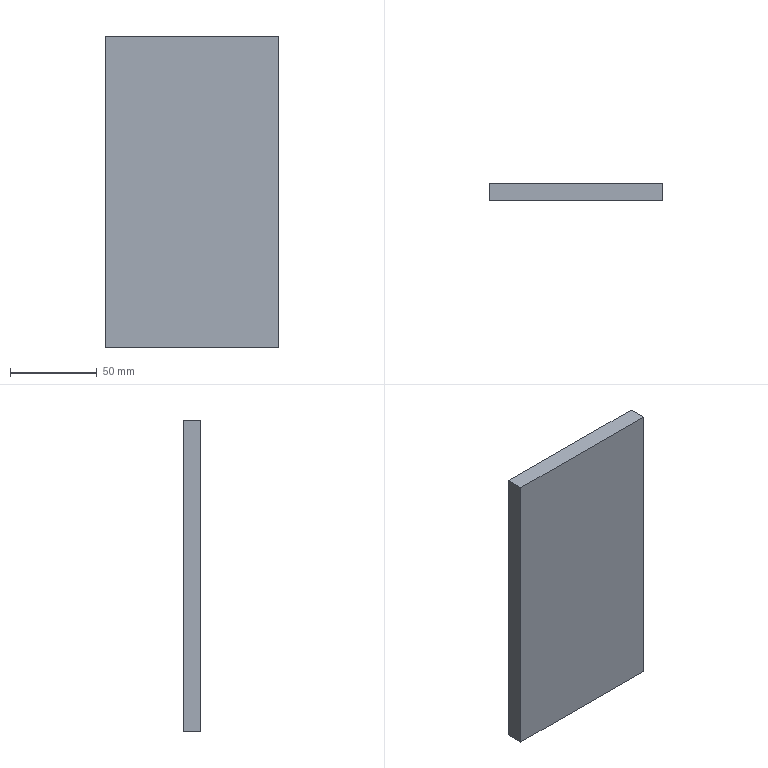Part | STEP file | A14-055 | 1 solid | 6 faces | box 100 x 10 x 180 mm | volume 180000 mm3 | plane 6
STEP:
#1=CARTESIAN_POINT('',(0.,0.,0.));
#2=DIRECTION('',(0.,0.,1.));
#3=DIRECTION('',(1.,0.,0.));
#4=AXIS2_PLACEMENT_3D('',#1,#2,#3);
#5=CARTESIAN_POINT('',(50.,-5.,90.));
#6=VERTEX_POINT('',#5);
#7=CARTESIAN_POINT('',(50.,-5.,-90.));
#8=VERTEX_POINT('',#7);
#9=CARTESIAN_POINT('',(50.,-5.,-90.));
#10=DIRECTION('',(0.,0.,-1.));
#11=VECTOR('',#10,1.);
#12=LINE('',#9,#11);
#13=CARTESIAN_POINT('',(50.,5.,-90.));
#14=DIRECTION('',(-1.,0.,0.));
#15=DIRECTION('',(0.,0.,1.));
#16=AXIS2_PLACEMENT_3D('',#13,#14,#15);
#17=PLANE('',#16);
#18=CARTESIAN_POINT('',(0.,-10.));
#19=DIRECTION('',(-1.,0.));
#20=VECTOR('',#19,1.);
#21=LINE('',#18,#20);
#22=(GEOMETRIC_REPRESENTATION_CONTEXT(2)PARAMETRIC_REPRESENTATION_CONTEXT()REPRESENTATION_CONTEXT('',''));
#23=DEFINITIONAL_REPRESENTATION('',(#21),#22);
#24=PCURVE('',#17,#23);
#25=CARTESIAN_POINT('',(0.,-5.,0.));
#26=DIRECTION('',(0.,1.,0.));
#27=DIRECTION('',(0.,0.,1.));
#28=AXIS2_PLACEMENT_3D('',#25,#26,#27);
#29=PLANE('',#28);
#30=CARTESIAN_POINT('',(-90.,50.));
#31=DIRECTION('',(-1.,0.));
#32=VECTOR('',#31,1.);
#33=LINE('',#30,#32);
#34=(GEOMETRIC_REPRESENTATION_CONTEXT(2)PARAMETRIC_REPRESENTATION_CONTEXT()REPRESENTATION_CONTEXT('',''));
#35=DEFINITIONAL_REPRESENTATION('',(#33),#34);
#36=PCURVE('',#29,#35);
#37=SURFACE_CURVE('',#12,(#24,#36),.PCURVE_S1.);
#38=EDGE_CURVE('',#6,#8,#37,.T.);
#39=ORIENTED_EDGE('',*,*,#38,.T.);
#40=CARTESIAN_POINT('',(50.,5.,-90.));
#41=VERTEX_POINT('',#40);
#42=CARTESIAN_POINT('',(50.,5.,-90.));
#43=DIRECTION('',(0.,-1.,0.));
#44=VECTOR('',#43,1.);
#45=LINE('',#42,#44);
#46=CARTESIAN_POINT('',(0.,0.));
#47=DIRECTION('',(0.,-1.));
#48=VECTOR('',#47,1.);
#49=LINE('',#46,#48);
#50=(GEOMETRIC_REPRESENTATION_CONTEXT(2)PARAMETRIC_REPRESENTATION_CONTEXT()REPRESENTATION_CONTEXT('',''));
#51=DEFINITIONAL_REPRESENTATION('',(#49),#50);
#52=PCURVE('',#17,#51);
#53=CARTESIAN_POINT('',(-50.,5.,-90.));
#54=DIRECTION('',(0.,0.,1.));
#55=DIRECTION('',(1.,0.,0.));
#56=AXIS2_PLACEMENT_3D('',#53,#54,#55);
#57=PLANE('',#56);
#58=CARTESIAN_POINT('',(100.,0.));
#59=DIRECTION('',(0.,-1.));
#60=VECTOR('',#59,1.);
#61=LINE('',#58,#60);
#62=(GEOMETRIC_REPRESENTATION_CONTEXT(2)PARAMETRIC_REPRESENTATION_CONTEXT()REPRESENTATION_CONTEXT('',''));
#63=DEFINITIONAL_REPRESENTATION('',(#61),#62);
#64=PCURVE('',#57,#63);
#65=SURFACE_CURVE('',#45,(#52,#64),.PCURVE_S1.);
#66=EDGE_CURVE('',#41,#8,#65,.T.);
#67=ORIENTED_EDGE('',*,*,#66,.F.);
#68=CARTESIAN_POINT('',(50.,5.,90.));
#69=VERTEX_POINT('',#68);
#70=CARTESIAN_POINT('',(50.,5.,-90.));
#71=DIRECTION('',(0.,0.,-1.));
#72=VECTOR('',#71,1.);
#73=LINE('',#70,#72);
#74=CARTESIAN_POINT('',(0.,0.));
#75=DIRECTION('',(-1.,0.));
#76=VECTOR('',#75,1.);
#77=LINE('',#74,#76);
#78=(GEOMETRIC_REPRESENTATION_CONTEXT(2)PARAMETRIC_REPRESENTATION_CONTEXT()REPRESENTATION_CONTEXT('',''));
#79=DEFINITIONAL_REPRESENTATION('',(#77),#78);
#80=PCURVE('',#17,#79);
#81=CARTESIAN_POINT('',(0.,5.,0.));
#82=DIRECTION('',(0.,1.,0.));
#83=DIRECTION('',(0.,0.,1.));
#84=AXIS2_PLACEMENT_3D('',#81,#82,#83);
#85=PLANE('',#84);
#86=CARTESIAN_POINT('',(-90.,50.));
#87=DIRECTION('',(-1.,0.));
#88=VECTOR('',#87,1.);
#89=LINE('',#86,#88);
#90=(GEOMETRIC_REPRESENTATION_CONTEXT(2)PARAMETRIC_REPRESENTATION_CONTEXT()REPRESENTATION_CONTEXT('',''));
#91=DEFINITIONAL_REPRESENTATION('',(#89),#90);
#92=PCURVE('',#85,#91);
#93=SURFACE_CURVE('',#73,(#80,#92),.PCURVE_S1.);
#94=EDGE_CURVE('',#69,#41,#93,.T.);
#95=ORIENTED_EDGE('',*,*,#94,.F.);
#96=CARTESIAN_POINT('',(50.,5.,90.));
#97=DIRECTION('',(0.,-1.,0.));
#98=VECTOR('',#97,1.);
#99=LINE('',#96,#98);
#100=CARTESIAN_POINT('',(180.,0.));
#101=DIRECTION('',(0.,-1.));
#102=VECTOR('',#101,1.);
#103=LINE('',#100,#102);
#104=(GEOMETRIC_REPRESENTATION_CONTEXT(2)PARAMETRIC_REPRESENTATION_CONTEXT()REPRESENTATION_CONTEXT('',''));
#105=DEFINITIONAL_REPRESENTATION('',(#103),#104);
#106=PCURVE('',#17,#105);
#107=CARTESIAN_POINT('',(-50.,5.,90.));
#108=DIRECTION('',(0.,0.,-1.));
#109=DIRECTION('',(-1.,0.,0.));
#110=AXIS2_PLACEMENT_3D('',#107,#108,#109);
#111=PLANE('',#110);
#112=CARTESIAN_POINT('',(-100.,0.));
#113=DIRECTION('',(0.,-1.));
#114=VECTOR('',#113,1.);
#115=LINE('',#112,#114);
#116=(GEOMETRIC_REPRESENTATION_CONTEXT(2)PARAMETRIC_REPRESENTATION_CONTEXT()REPRESENTATION_CONTEXT('',''));
#117=DEFINITIONAL_REPRESENTATION('',(#115),#116);
#118=PCURVE('',#111,#117);
#119=SURFACE_CURVE('',#99,(#106,#118),.PCURVE_S1.);
#120=EDGE_CURVE('',#69,#6,#119,.T.);
#121=ORIENTED_EDGE('',*,*,#120,.T.);
#122=EDGE_LOOP('',(#39,#67,#95,#121));
#123=FACE_BOUND('',#122,.T.);
#124=ADVANCED_FACE('',(#123),#17,.F.);
#125=CARTESIAN_POINT('',(-50.,-5.,-90.));
#126=VERTEX_POINT('',#125);
#127=CARTESIAN_POINT('',(-50.,-5.,-90.));
#128=DIRECTION('',(-1.,0.,0.));
#129=VECTOR('',#128,1.);
#130=LINE('',#127,#129);
#131=CARTESIAN_POINT('',(0.,-10.));
#132=DIRECTION('',(-1.,0.));
#133=VECTOR('',#132,1.);
#134=LINE('',#131,#133);
#135=(GEOMETRIC_REPRESENTATION_CONTEXT(2)PARAMETRIC_REPRESENTATION_CONTEXT()REPRESENTATION_CONTEXT('',''));
#136=DEFINITIONAL_REPRESENTATION('',(#134),#135);
#137=PCURVE('',#57,#136);
#138=CARTESIAN_POINT('',(-90.,-50.));
#139=DIRECTION('',(0.,-1.));
#140=VECTOR('',#139,1.);
#141=LINE('',#138,#140);
#142=(GEOMETRIC_REPRESENTATION_CONTEXT(2)PARAMETRIC_REPRESENTATION_CONTEXT()REPRESENTATION_CONTEXT('',''));
#143=DEFINITIONAL_REPRESENTATION('',(#141),#142);
#144=PCURVE('',#29,#143);
#145=SURFACE_CURVE('',#130,(#137,#144),.PCURVE_S1.);
#146=EDGE_CURVE('',#8,#126,#145,.T.);
#147=ORIENTED_EDGE('',*,*,#146,.T.);
#148=CARTESIAN_POINT('',(-50.,5.,-90.));
#149=VERTEX_POINT('',#148);
#150=CARTESIAN_POINT('',(-50.,5.,-90.));
#151=DIRECTION('',(0.,-1.,0.));
#152=VECTOR('',#151,1.);
#153=LINE('',#150,#152);
#154=CARTESIAN_POINT('',(0.,0.));
#155=DIRECTION('',(0.,-1.));
#156=VECTOR('',#155,1.);
#157=LINE('',#154,#156);
#158=(GEOMETRIC_REPRESENTATION_CONTEXT(2)PARAMETRIC_REPRESENTATION_CONTEXT()REPRESENTATION_CONTEXT('',''));
#159=DEFINITIONAL_REPRESENTATION('',(#157),#158);
#160=PCURVE('',#57,#159);
#161=CARTESIAN_POINT('',(-50.,5.,-90.));
#162=DIRECTION('',(1.,0.,0.));
#163=DIRECTION('',(0.,0.,-1.));
#164=AXIS2_PLACEMENT_3D('',#161,#162,#163);
#165=PLANE('',#164);
#166=CARTESIAN_POINT('',(0.,0.));
#167=DIRECTION('',(0.,-1.));
#168=VECTOR('',#167,1.);
#169=LINE('',#166,#168);
#170=(GEOMETRIC_REPRESENTATION_CONTEXT(2)PARAMETRIC_REPRESENTATION_CONTEXT()REPRESENTATION_CONTEXT('',''));
#171=DEFINITIONAL_REPRESENTATION('',(#169),#170);
#172=PCURVE('',#165,#171);
#173=SURFACE_CURVE('',#153,(#160,#172),.PCURVE_S1.);
#174=EDGE_CURVE('',#149,#126,#173,.T.);
#175=ORIENTED_EDGE('',*,*,#174,.F.);
#176=CARTESIAN_POINT('',(-50.,5.,-90.));
#177=DIRECTION('',(-1.,0.,0.));
#178=VECTOR('',#177,1.);
#179=LINE('',#176,#178);
#180=CARTESIAN_POINT('',(0.,0.));
#181=DIRECTION('',(-1.,0.));
#182=VECTOR('',#181,1.);
#183=LINE('',#180,#182);
#184=(GEOMETRIC_REPRESENTATION_CONTEXT(2)PARAMETRIC_REPRESENTATION_CONTEXT()REPRESENTATION_CONTEXT('',''));
#185=DEFINITIONAL_REPRESENTATION('',(#183),#184);
#186=PCURVE('',#57,#185);
#187=CARTESIAN_POINT('',(-90.,-50.));
#188=DIRECTION('',(0.,-1.));
#189=VECTOR('',#188,1.);
#190=LINE('',#187,#189);
#191=(GEOMETRIC_REPRESENTATION_CONTEXT(2)PARAMETRIC_REPRESENTATION_CONTEXT()REPRESENTATION_CONTEXT('',''));
#192=DEFINITIONAL_REPRESENTATION('',(#190),#191);
#193=PCURVE('',#85,#192);
#194=SURFACE_CURVE('',#179,(#186,#193),.PCURVE_S1.);
#195=EDGE_CURVE('',#41,#149,#194,.T.);
#196=ORIENTED_EDGE('',*,*,#195,.F.);
#197=ORIENTED_EDGE('',*,*,#66,.T.);
#198=EDGE_LOOP('',(#147,#175,#196,#197));
#199=FACE_BOUND('',#198,.T.);
#200=ADVANCED_FACE('',(#199),#57,.F.);
#201=CARTESIAN_POINT('',(-50.,-5.,90.));
#202=VERTEX_POINT('',#201);
#203=CARTESIAN_POINT('',(-50.,-5.,-90.));
#204=DIRECTION('',(0.,0.,1.));
#205=VECTOR('',#204,1.);
#206=LINE('',#203,#205);
#207=CARTESIAN_POINT('',(0.,-10.));
#208=DIRECTION('',(-1.,0.));
#209=VECTOR('',#208,1.);
#210=LINE('',#207,#209);
#211=(GEOMETRIC_REPRESENTATION_CONTEXT(2)PARAMETRIC_REPRESENTATION_CONTEXT()REPRESENTATION_CONTEXT('',''));
#212=DEFINITIONAL_REPRESENTATION('',(#210),#211);
#213=PCURVE('',#165,#212);
#214=CARTESIAN_POINT('',(-90.,-50.));
#215=DIRECTION('',(1.,0.));
#216=VECTOR('',#215,1.);
#217=LINE('',#214,#216);
#218=(GEOMETRIC_REPRESENTATION_CONTEXT(2)PARAMETRIC_REPRESENTATION_CONTEXT()REPRESENTATION_CONTEXT('',''));
#219=DEFINITIONAL_REPRESENTATION('',(#217),#218);
#220=PCURVE('',#29,#219);
#221=SURFACE_CURVE('',#206,(#213,#220),.PCURVE_S1.);
#222=EDGE_CURVE('',#126,#202,#221,.T.);
#223=ORIENTED_EDGE('',*,*,#222,.T.);
#224=CARTESIAN_POINT('',(-50.,5.,90.));
#225=VERTEX_POINT('',#224);
#226=CARTESIAN_POINT('',(-50.,5.,90.));
#227=DIRECTION('',(0.,-1.,0.));
#228=VECTOR('',#227,1.);
#229=LINE('',#226,#228);
#230=CARTESIAN_POINT('',(-180.,0.));
#231=DIRECTION('',(0.,-1.));
#232=VECTOR('',#231,1.);
#233=LINE('',#230,#232);
#234=(GEOMETRIC_REPRESENTATION_CONTEXT(2)PARAMETRIC_REPRESENTATION_CONTEXT()REPRESENTATION_CONTEXT('',''));
#235=DEFINITIONAL_REPRESENTATION('',(#233),#234);
#236=PCURVE('',#165,#235);
#237=CARTESIAN_POINT('',(0.,0.));
#238=DIRECTION('',(0.,-1.));
#239=VECTOR('',#238,1.);
#240=LINE('',#237,#239);
#241=(GEOMETRIC_REPRESENTATION_CONTEXT(2)PARAMETRIC_REPRESENTATION_CONTEXT()REPRESENTATION_CONTEXT('',''));
#242=DEFINITIONAL_REPRESENTATION('',(#240),#241);
#243=PCURVE('',#111,#242);
#244=SURFACE_CURVE('',#229,(#236,#243),.PCURVE_S1.);
#245=EDGE_CURVE('',#225,#202,#244,.T.);
#246=ORIENTED_EDGE('',*,*,#245,.F.);
#247=CARTESIAN_POINT('',(-50.,5.,-90.));
#248=DIRECTION('',(0.,0.,1.));
#249=VECTOR('',#248,1.);
#250=LINE('',#247,#249);
#251=CARTESIAN_POINT('',(0.,0.));
#252=DIRECTION('',(-1.,0.));
#253=VECTOR('',#252,1.);
#254=LINE('',#251,#253);
#255=(GEOMETRIC_REPRESENTATION_CONTEXT(2)PARAMETRIC_REPRESENTATION_CONTEXT()REPRESENTATION_CONTEXT('',''));
#256=DEFINITIONAL_REPRESENTATION('',(#254),#255);
#257=PCURVE('',#165,#256);
#258=CARTESIAN_POINT('',(-90.,-50.));
#259=DIRECTION('',(1.,0.));
#260=VECTOR('',#259,1.);
#261=LINE('',#258,#260);
#262=(GEOMETRIC_REPRESENTATION_CONTEXT(2)PARAMETRIC_REPRESENTATION_CONTEXT()REPRESENTATION_CONTEXT('',''));
#263=DEFINITIONAL_REPRESENTATION('',(#261),#262);
#264=PCURVE('',#85,#263);
#265=SURFACE_CURVE('',#250,(#257,#264),.PCURVE_S1.);
#266=EDGE_CURVE('',#149,#225,#265,.T.);
#267=ORIENTED_EDGE('',*,*,#266,.F.);
#268=ORIENTED_EDGE('',*,*,#174,.T.);
#269=EDGE_LOOP('',(#223,#246,#267,#268));
#270=FACE_BOUND('',#269,.T.);
#271=ADVANCED_FACE('',(#270),#165,.F.);
#272=CARTESIAN_POINT('',(-50.,-5.,90.));
#273=DIRECTION('',(1.,0.,0.));
#274=VECTOR('',#273,1.);
#275=LINE('',#272,#274);
#276=CARTESIAN_POINT('',(0.,-10.));
#277=DIRECTION('',(-1.,0.));
#278=VECTOR('',#277,1.);
#279=LINE('',#276,#278);
#280=(GEOMETRIC_REPRESENTATION_CONTEXT(2)PARAMETRIC_REPRESENTATION_CONTEXT()REPRESENTATION_CONTEXT('',''));
#281=DEFINITIONAL_REPRESENTATION('',(#279),#280);
#282=PCURVE('',#111,#281);
#283=CARTESIAN_POINT('',(90.,-50.));
#284=DIRECTION('',(0.,1.));
#285=VECTOR('',#284,1.);
#286=LINE('',#283,#285);
#287=(GEOMETRIC_REPRESENTATION_CONTEXT(2)PARAMETRIC_REPRESENTATION_CONTEXT()REPRESENTATION_CONTEXT('',''));
#288=DEFINITIONAL_REPRESENTATION('',(#286),#287);
#289=PCURVE('',#29,#288);
#290=SURFACE_CURVE('',#275,(#282,#289),.PCURVE_S1.);
#291=EDGE_CURVE('',#202,#6,#290,.T.);
#292=ORIENTED_EDGE('',*,*,#291,.T.);
#293=ORIENTED_EDGE('',*,*,#120,.F.);
#294=CARTESIAN_POINT('',(-50.,5.,90.));
#295=DIRECTION('',(1.,0.,0.));
#296=VECTOR('',#295,1.);
#297=LINE('',#294,#296);
#298=CARTESIAN_POINT('',(0.,0.));
#299=DIRECTION('',(-1.,0.));
#300=VECTOR('',#299,1.);
#301=LINE('',#298,#300);
#302=(GEOMETRIC_REPRESENTATION_CONTEXT(2)PARAMETRIC_REPRESENTATION_CONTEXT()REPRESENTATION_CONTEXT('',''));
#303=DEFINITIONAL_REPRESENTATION('',(#301),#302);
#304=PCURVE('',#111,#303);
#305=CARTESIAN_POINT('',(90.,-50.));
#306=DIRECTION('',(0.,1.));
#307=VECTOR('',#306,1.);
#308=LINE('',#305,#307);
#309=(GEOMETRIC_REPRESENTATION_CONTEXT(2)PARAMETRIC_REPRESENTATION_CONTEXT()REPRESENTATION_CONTEXT('',''));
#310=DEFINITIONAL_REPRESENTATION('',(#308),#309);
#311=PCURVE('',#85,#310);
#312=SURFACE_CURVE('',#297,(#304,#311),.PCURVE_S1.);
#313=EDGE_CURVE('',#225,#69,#312,.T.);
#314=ORIENTED_EDGE('',*,*,#313,.F.);
#315=ORIENTED_EDGE('',*,*,#245,.T.);
#316=EDGE_LOOP('',(#292,#293,#314,#315));
#317=FACE_BOUND('',#316,.T.);
#318=ADVANCED_FACE('',(#317),#111,.F.);
#319=ORIENTED_EDGE('',*,*,#94,.T.);
#320=ORIENTED_EDGE('',*,*,#195,.T.);
#321=ORIENTED_EDGE('',*,*,#266,.T.);
#322=ORIENTED_EDGE('',*,*,#313,.T.);
#323=EDGE_LOOP('',(#319,#320,#321,#322));
#324=FACE_BOUND('',#323,.T.);
#325=ADVANCED_FACE('',(#324),#85,.T.);
#326=ORIENTED_EDGE('',*,*,#38,.F.);
#327=ORIENTED_EDGE('',*,*,#291,.F.);
#328=ORIENTED_EDGE('',*,*,#222,.F.);
#329=ORIENTED_EDGE('',*,*,#146,.F.);
#330=EDGE_LOOP('',(#326,#327,#328,#329));
#331=FACE_BOUND('',#330,.T.);
#332=ADVANCED_FACE('',(#331),#29,.F.);
#333=CLOSED_SHELL('',(#124,#200,#271,#318,#325,#332));
#334=MANIFOLD_SOLID_BREP('',#333);
#335=(LENGTH_UNIT()NAMED_UNIT(*)SI_UNIT(.MILLI.,.METRE.));
#336=UNCERTAINTY_MEASURE_WITH_UNIT(LENGTH_MEASURE(0.0000001),#335,'','');
#337=(NAMED_UNIT(*)PLANE_ANGLE_UNIT()SI_UNIT($,.RADIAN.));
#338=(NAMED_UNIT(*)SI_UNIT($,.STERADIAN.)SOLID_ANGLE_UNIT());
#339=(GEOMETRIC_REPRESENTATION_CONTEXT(3)GLOBAL_UNCERTAINTY_ASSIGNED_CONTEXT((#336))GLOBAL_UNIT_ASSIGNED_CONTEXT((#335,#337,#338))REPRESENTATION_CONTEXT('',''));
#340=ADVANCED_BREP_SHAPE_REPRESENTATION('',(#4,#334),#339);